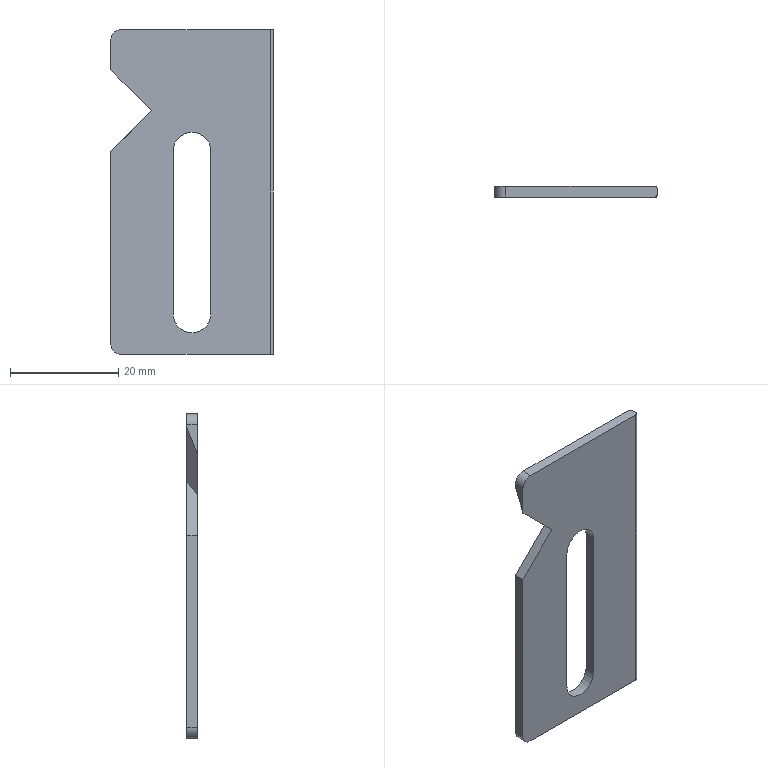Part | SolidWorks | features BaseBody 1 | 1 solid | 18 faces | box 30 x 2 x 60 mm | volume 2939 mm3 | plane 11 | cylinder 7 | commonest cylinder face diameters 7 x3 1 x2 4 x2
STEP:
#1=CARTESIAN_POINT('',(-11.5,0.,-22.5));
#2=VERTEX_POINT('',#1);
#3=CARTESIAN_POINT('',(-15.,0.,-19.));
#4=VERTEX_POINT('',#3);
#5=CARTESIAN_POINT('',(-15.,0.,-22.5));
#6=DIRECTION('',(0.,-1.,0.));
#7=DIRECTION('',(0.,0.,1.));
#8=AXIS2_PLACEMENT_3D('',#5,#6,#7);
#9=CIRCLE('',#8,3.5);
#10=EDGE_CURVE('',#2,#4,#9,.T.);
#11=ORIENTED_EDGE('',*,*,#10,.T.);
#12=CARTESIAN_POINT('',(-15.,2.,-19.));
#13=VERTEX_POINT('',#12);
#14=CARTESIAN_POINT('',(-15.,-8.,-19.));
#15=DIRECTION('',(0.,1.,0.));
#16=VECTOR('',#15,1000.);
#17=LINE('',#14,#16);
#18=EDGE_CURVE('',#4,#13,#17,.T.);
#19=ORIENTED_EDGE('',*,*,#18,.T.);
#20=CARTESIAN_POINT('',(-11.5,2.,-22.5));
#21=VERTEX_POINT('',#20);
#22=CARTESIAN_POINT('',(-15.,2.,-22.5));
#23=DIRECTION('',(0.,-1.,0.));
#24=DIRECTION('',(0.,0.,1.));
#25=AXIS2_PLACEMENT_3D('',#22,#23,#24);
#26=CIRCLE('',#25,3.5);
#27=EDGE_CURVE('',#21,#13,#26,.T.);
#28=ORIENTED_EDGE('',*,*,#27,.F.);
#29=CARTESIAN_POINT('',(-11.5,-8.,-22.5));
#30=DIRECTION('',(0.,1.,0.));
#31=VECTOR('',#30,1000.);
#32=LINE('',#29,#31);
#33=EDGE_CURVE('',#2,#21,#32,.T.);
#34=ORIENTED_EDGE('',*,*,#33,.F.);
#35=EDGE_LOOP('',(#11,#19,#28,#34));
#36=FACE_OUTER_BOUND('',#35,.T.);
#37=CARTESIAN_POINT('',(-15.,-8.,-22.5));
#38=DIRECTION('',(0.,1.,0.));
#39=DIRECTION('',(0.,0.,1.));
#40=AXIS2_PLACEMENT_3D('',#37,#38,#39);
#41=CYLINDRICAL_SURFACE('',#40,3.5);
#42=ADVANCED_FACE('',(#36),#41,.F.);
#43=CARTESIAN_POINT('',(-30.,0.,-22.5));
#44=VERTEX_POINT('',#43);
#45=CARTESIAN_POINT('',(-22.475,0.,-14.975));
#46=VERTEX_POINT('',#45);
#47=CARTESIAN_POINT('',(-30.,0.,-22.5));
#48=DIRECTION('',(0.7071,0.,0.7071));
#49=VECTOR('',#48,1000.);
#50=LINE('',#47,#49);
#51=EDGE_CURVE('',#44,#46,#50,.T.);
#52=ORIENTED_EDGE('',*,*,#51,.F.);
#53=CARTESIAN_POINT('',(-30.,0.,-58.));
#54=VERTEX_POINT('',#53);
#55=CARTESIAN_POINT('',(-30.,0.,-60.));
#56=DIRECTION('',(0.,0.,1.));
#57=VECTOR('',#56,1000.);
#58=LINE('',#55,#57);
#59=EDGE_CURVE('',#54,#44,#58,.T.);
#60=ORIENTED_EDGE('',*,*,#59,.F.);
#61=CARTESIAN_POINT('',(-28.,0.,-60.));
#62=VERTEX_POINT('',#61);
#63=CARTESIAN_POINT('',(-28.,0.,-58.));
#64=DIRECTION('',(0.,1.,0.));
#65=DIRECTION('',(0.,0.,-1.));
#66=AXIS2_PLACEMENT_3D('',#63,#64,#65);
#67=CIRCLE('',#66,2.);
#68=EDGE_CURVE('',#62,#54,#67,.T.);
#69=ORIENTED_EDGE('',*,*,#68,.F.);
#70=CARTESIAN_POINT('',(-0.5,0.,-60.));
#71=VERTEX_POINT('',#70);
#72=CARTESIAN_POINT('',(0.,0.,-60.));
#73=DIRECTION('',(-1.,0.,0.));
#74=VECTOR('',#73,1000.);
#75=LINE('',#72,#74);
#76=EDGE_CURVE('',#71,#62,#75,.T.);
#77=ORIENTED_EDGE('',*,*,#76,.F.);
#78=CARTESIAN_POINT('',(-0.5,0.,0.));
#79=VERTEX_POINT('',#78);
#80=CARTESIAN_POINT('',(-0.5,0.,-60.));
#81=DIRECTION('',(0.,0.,-1.));
#82=VECTOR('',#81,1000.);
#83=LINE('',#80,#82);
#84=EDGE_CURVE('',#79,#71,#83,.T.);
#85=ORIENTED_EDGE('',*,*,#84,.F.);
#86=CARTESIAN_POINT('',(-28.,0.,0.));
#87=VERTEX_POINT('',#86);
#88=CARTESIAN_POINT('',(0.,0.,0.));
#89=DIRECTION('',(1.,0.,0.));
#90=VECTOR('',#89,1000.);
#91=LINE('',#88,#90);
#92=EDGE_CURVE('',#87,#79,#91,.T.);
#93=ORIENTED_EDGE('',*,*,#92,.F.);
#94=CARTESIAN_POINT('',(-30.,0.,-2.));
#95=VERTEX_POINT('',#94);
#96=CARTESIAN_POINT('',(-28.,0.,-2.));
#97=DIRECTION('',(0.,1.,0.));
#98=DIRECTION('',(0.,0.,-1.));
#99=AXIS2_PLACEMENT_3D('',#96,#97,#98);
#100=CIRCLE('',#99,2.);
#101=EDGE_CURVE('',#95,#87,#100,.T.);
#102=ORIENTED_EDGE('',*,*,#101,.F.);
#103=CARTESIAN_POINT('',(-30.,0.,-7.449));
#104=VERTEX_POINT('',#103);
#105=CARTESIAN_POINT('',(-30.,0.,-60.));
#106=DIRECTION('',(0.,0.,1.));
#107=VECTOR('',#106,1000.);
#108=LINE('',#105,#107);
#109=EDGE_CURVE('',#104,#95,#108,.T.);
#110=ORIENTED_EDGE('',*,*,#109,.F.);
#111=CARTESIAN_POINT('',(-22.475,0.,-14.975));
#112=DIRECTION('',(-0.7071,0.,0.7071));
#113=VECTOR('',#112,1000.);
#114=LINE('',#111,#113);
#115=EDGE_CURVE('',#46,#104,#114,.T.);
#116=ORIENTED_EDGE('',*,*,#115,.F.);
#117=EDGE_LOOP('',(#52,#60,#69,#77,#85,#93,#102,#110,#116));
#118=FACE_OUTER_BOUND('',#117,.T.);
#119=CARTESIAN_POINT('',(-18.5,0.,-22.5));
#120=VERTEX_POINT('',#119);
#121=CARTESIAN_POINT('',(-18.5,0.,-52.5));
#122=VERTEX_POINT('',#121);
#123=CARTESIAN_POINT('',(-18.5,0.,-60.));
#124=DIRECTION('',(0.,0.,-1.));
#125=VECTOR('',#124,1000.);
#126=LINE('',#123,#125);
#127=EDGE_CURVE('',#120,#122,#126,.T.);
#128=ORIENTED_EDGE('',*,*,#127,.F.);
#129=CARTESIAN_POINT('',(-15.,0.,-22.5));
#130=DIRECTION('',(0.,-1.,0.));
#131=DIRECTION('',(0.,0.,1.));
#132=AXIS2_PLACEMENT_3D('',#129,#130,#131);
#133=CIRCLE('',#132,3.5);
#134=EDGE_CURVE('',#4,#120,#133,.T.);
#135=ORIENTED_EDGE('',*,*,#134,.F.);
#136=ORIENTED_EDGE('',*,*,#10,.F.);
#137=CARTESIAN_POINT('',(-11.5,0.,-52.5));
#138=VERTEX_POINT('',#137);
#139=CARTESIAN_POINT('',(-11.5,0.,-60.));
#140=DIRECTION('',(0.,0.,1.));
#141=VECTOR('',#140,1000.);
#142=LINE('',#139,#141);
#143=EDGE_CURVE('',#138,#2,#142,.T.);
#144=ORIENTED_EDGE('',*,*,#143,.F.);
#145=CARTESIAN_POINT('',(-15.,0.,-52.5));
#146=DIRECTION('',(0.,-1.,0.));
#147=DIRECTION('',(0.,0.,1.));
#148=AXIS2_PLACEMENT_3D('',#145,#146,#147);
#149=CIRCLE('',#148,3.5);
#150=EDGE_CURVE('',#122,#138,#149,.T.);
#151=ORIENTED_EDGE('',*,*,#150,.F.);
#152=EDGE_LOOP('',(#128,#135,#136,#144,#151));
#153=FACE_BOUND('',#152,.T.);
#154=CARTESIAN_POINT('',(0.,0.,-60.));
#155=DIRECTION('',(0.,1.,0.));
#156=DIRECTION('',(0.,0.,1.));
#157=AXIS2_PLACEMENT_3D('',#154,#155,#156);
#158=PLANE('',#157);
#159=ADVANCED_FACE('',(#118,#153),#158,.F.);
#160=CARTESIAN_POINT('',(-20.025,2.,-12.525));
#161=VERTEX_POINT('',#160);
#162=CARTESIAN_POINT('',(-20.025,2.,-12.525));
#163=DIRECTION('',(-0.6124,-0.5,-0.6124));
#164=VECTOR('',#163,1000.);
#165=LINE('',#162,#164);
#166=EDGE_CURVE('',#161,#46,#165,.T.);
#167=ORIENTED_EDGE('',*,*,#166,.T.);
#168=ORIENTED_EDGE('',*,*,#115,.T.);
#169=CARTESIAN_POINT('',(-30.,2.,-2.55));
#170=VERTEX_POINT('',#169);
#171=CARTESIAN_POINT('',(-30.,-2.645,-13.929));
#172=DIRECTION('',(0.,0.378,0.9258));
#173=VECTOR('',#172,1000.);
#174=LINE('',#171,#173);
#175=EDGE_CURVE('',#104,#170,#174,.T.);
#176=ORIENTED_EDGE('',*,*,#175,.T.);
#177=CARTESIAN_POINT('',(-30.,2.,-2.55));
#178=DIRECTION('',(0.7071,0.,-0.7071));
#179=VECTOR('',#178,1000.);
#180=LINE('',#177,#179);
#181=EDGE_CURVE('',#170,#161,#180,.T.);
#182=ORIENTED_EDGE('',*,*,#181,.T.);
#183=EDGE_LOOP('',(#167,#168,#176,#182));
#184=FACE_OUTER_BOUND('',#183,.T.);
#185=CARTESIAN_POINT('',(-22.5,-0.02073,-15.));
#186=DIRECTION('',(-0.3536,0.866,-0.3536));
#187=DIRECTION('',(0.,0.378,0.9258));
#188=AXIS2_PLACEMENT_3D('',#185,#186,#187);
#189=PLANE('',#188);
#190=ADVANCED_FACE('',(#184),#189,.T.);
#191=CARTESIAN_POINT('',(-30.,2.,-22.5));
#192=VERTEX_POINT('',#191);
#193=CARTESIAN_POINT('',(-30.,10.,-22.5));
#194=DIRECTION('',(0.,1.,0.));
#195=VECTOR('',#194,1000.);
#196=LINE('',#193,#195);
#197=EDGE_CURVE('',#44,#192,#196,.T.);
#198=ORIENTED_EDGE('',*,*,#197,.F.);
#199=ORIENTED_EDGE('',*,*,#51,.T.);
#200=ORIENTED_EDGE('',*,*,#166,.F.);
#201=CARTESIAN_POINT('',(-30.,2.,-22.5));
#202=DIRECTION('',(0.7071,0.,0.7071));
#203=VECTOR('',#202,1000.);
#204=LINE('',#201,#203);
#205=EDGE_CURVE('',#192,#161,#204,.T.);
#206=ORIENTED_EDGE('',*,*,#205,.F.);
#207=EDGE_LOOP('',(#198,#199,#200,#206));
#208=FACE_OUTER_BOUND('',#207,.T.);
#209=CARTESIAN_POINT('',(-30.,10.,-22.5));
#210=DIRECTION('',(0.7071,0.,-0.7071));
#211=DIRECTION('',(-0.7071,0.,-0.7071));
#212=AXIS2_PLACEMENT_3D('',#209,#210,#211);
#213=PLANE('',#212);
#214=ADVANCED_FACE('',(#208),#213,.F.);
#215=CARTESIAN_POINT('',(-30.,2.,-58.));
#216=VERTEX_POINT('',#215);
#217=CARTESIAN_POINT('',(-30.,2.,-58.));
#218=DIRECTION('',(0.,1.,0.));
#219=VECTOR('',#218,1000.);
#220=LINE('',#217,#219);
#221=EDGE_CURVE('',#54,#216,#220,.T.);
#222=ORIENTED_EDGE('',*,*,#221,.F.);
#223=ORIENTED_EDGE('',*,*,#59,.T.);
#224=ORIENTED_EDGE('',*,*,#197,.T.);
#225=CARTESIAN_POINT('',(-30.,2.,0.));
#226=DIRECTION('',(0.,0.,1.));
#227=VECTOR('',#226,1000.);
#228=LINE('',#225,#227);
#229=EDGE_CURVE('',#216,#192,#228,.T.);
#230=ORIENTED_EDGE('',*,*,#229,.F.);
#231=EDGE_LOOP('',(#222,#223,#224,#230));
#232=FACE_OUTER_BOUND('',#231,.T.);
#233=CARTESIAN_POINT('',(-30.,2.,0.));
#234=DIRECTION('',(1.,0.,0.));
#235=DIRECTION('',(0.,0.,-1.));
#236=AXIS2_PLACEMENT_3D('',#233,#234,#235);
#237=PLANE('',#236);
#238=ADVANCED_FACE('',(#232),#237,.F.);
#239=ORIENTED_EDGE('',*,*,#68,.T.);
#240=ORIENTED_EDGE('',*,*,#221,.T.);
#241=CARTESIAN_POINT('',(-28.,2.,-60.));
#242=VERTEX_POINT('',#241);
#243=CARTESIAN_POINT('',(-28.,2.,-58.));
#244=DIRECTION('',(0.,-1.,0.));
#245=DIRECTION('',(0.,0.,-1.));
#246=AXIS2_PLACEMENT_3D('',#243,#244,#245);
#247=CIRCLE('',#246,2.);
#248=EDGE_CURVE('',#216,#242,#247,.T.);
#249=ORIENTED_EDGE('',*,*,#248,.T.);
#250=CARTESIAN_POINT('',(-28.,2.,-60.));
#251=DIRECTION('',(0.,-1.,0.));
#252=VECTOR('',#251,1000.);
#253=LINE('',#250,#252);
#254=EDGE_CURVE('',#242,#62,#253,.T.);
#255=ORIENTED_EDGE('',*,*,#254,.T.);
#256=EDGE_LOOP('',(#239,#240,#249,#255));
#257=FACE_OUTER_BOUND('',#256,.T.);
#258=CARTESIAN_POINT('',(-28.,2.,-58.));
#259=DIRECTION('',(0.,-1.,0.));
#260=DIRECTION('',(0.,0.,-1.));
#261=AXIS2_PLACEMENT_3D('',#258,#259,#260);
#262=CYLINDRICAL_SURFACE('',#261,2.);
#263=ADVANCED_FACE('',(#257),#262,.T.);
#264=ORIENTED_EDGE('',*,*,#254,.F.);
#265=CARTESIAN_POINT('',(-0.5,2.,-60.));
#266=VERTEX_POINT('',#265);
#267=CARTESIAN_POINT('',(0.,2.,-60.));
#268=DIRECTION('',(-1.,0.,0.));
#269=VECTOR('',#268,1000.);
#270=LINE('',#267,#269);
#271=EDGE_CURVE('',#266,#242,#270,.T.);
#272=ORIENTED_EDGE('',*,*,#271,.F.);
#273=CARTESIAN_POINT('',(0.,1.5,-60.));
#274=VERTEX_POINT('',#273);
#275=CARTESIAN_POINT('',(-0.5,1.5,-60.));
#276=DIRECTION('',(0.,0.,1.));
#277=DIRECTION('',(1.,0.,0.));
#278=AXIS2_PLACEMENT_3D('',#275,#276,#277);
#279=CIRCLE('',#278,0.5);
#280=EDGE_CURVE('',#274,#266,#279,.T.);
#281=ORIENTED_EDGE('',*,*,#280,.F.);
#282=CARTESIAN_POINT('',(0.,0.5,-60.));
#283=VERTEX_POINT('',#282);
#284=CARTESIAN_POINT('',(0.,2.,-60.));
#285=DIRECTION('',(0.,-1.,0.));
#286=VECTOR('',#285,1000.);
#287=LINE('',#284,#286);
#288=EDGE_CURVE('',#274,#283,#287,.T.);
#289=ORIENTED_EDGE('',*,*,#288,.T.);
#290=CARTESIAN_POINT('',(-0.5,0.5,-60.));
#291=DIRECTION('',(0.,0.,1.));
#292=DIRECTION('',(-1.,0.,0.));
#293=AXIS2_PLACEMENT_3D('',#290,#291,#292);
#294=CIRCLE('',#293,0.5);
#295=EDGE_CURVE('',#71,#283,#294,.T.);
#296=ORIENTED_EDGE('',*,*,#295,.F.);
#297=ORIENTED_EDGE('',*,*,#76,.T.);
#298=EDGE_LOOP('',(#264,#272,#281,#289,#296,#297));
#299=FACE_OUTER_BOUND('',#298,.T.);
#300=CARTESIAN_POINT('',(0.,2.,-60.));
#301=DIRECTION('',(0.,0.,1.));
#302=DIRECTION('',(1.,0.,0.));
#303=AXIS2_PLACEMENT_3D('',#300,#301,#302);
#304=PLANE('',#303);
#305=ADVANCED_FACE('',(#299),#304,.F.);
#306=ORIENTED_EDGE('',*,*,#295,.T.);
#307=CARTESIAN_POINT('',(0.,0.5,0.));
#308=VERTEX_POINT('',#307);
#309=CARTESIAN_POINT('',(0.,0.5,0.));
#310=DIRECTION('',(0.,0.,1.));
#311=VECTOR('',#310,1000.);
#312=LINE('',#309,#311);
#313=EDGE_CURVE('',#283,#308,#312,.T.);
#314=ORIENTED_EDGE('',*,*,#313,.T.);
#315=CARTESIAN_POINT('',(-0.5,0.5,0.));
#316=DIRECTION('',(0.,0.,-1.));
#317=DIRECTION('',(-1.,0.,0.));
#318=AXIS2_PLACEMENT_3D('',#315,#316,#317);
#319=CIRCLE('',#318,0.5);
#320=EDGE_CURVE('',#308,#79,#319,.T.);
#321=ORIENTED_EDGE('',*,*,#320,.T.);
#322=ORIENTED_EDGE('',*,*,#84,.T.);
#323=EDGE_LOOP('',(#306,#314,#321,#322));
#324=FACE_OUTER_BOUND('',#323,.T.);
#325=CARTESIAN_POINT('',(-0.5,0.5,0.));
#326=DIRECTION('',(0.,0.,-1.));
#327=DIRECTION('',(-1.,0.,0.));
#328=AXIS2_PLACEMENT_3D('',#325,#326,#327);
#329=CYLINDRICAL_SURFACE('',#328,0.5);
#330=ADVANCED_FACE('',(#324),#329,.T.);
#331=CARTESIAN_POINT('',(-28.,2.,0.));
#332=VERTEX_POINT('',#331);
#333=CARTESIAN_POINT('',(-28.,2.,0.));
#334=DIRECTION('',(0.,1.,0.));
#335=VECTOR('',#334,1000.);
#336=LINE('',#333,#335);
#337=EDGE_CURVE('',#87,#332,#336,.T.);
#338=ORIENTED_EDGE('',*,*,#337,.F.);
#339=ORIENTED_EDGE('',*,*,#92,.T.);
#340=ORIENTED_EDGE('',*,*,#320,.F.);
#341=CARTESIAN_POINT('',(0.,1.5,0.));
#342=VERTEX_POINT('',#341);
#343=CARTESIAN_POINT('',(0.,2.,0.));
#344=DIRECTION('',(0.,-1.,0.));
#345=VECTOR('',#344,1000.);
#346=LINE('',#343,#345);
#347=EDGE_CURVE('',#342,#308,#346,.T.);
#348=ORIENTED_EDGE('',*,*,#347,.F.);
#349=CARTESIAN_POINT('',(-0.5,2.,0.));
#350=VERTEX_POINT('',#349);
#351=CARTESIAN_POINT('',(-0.5,1.5,0.));
#352=DIRECTION('',(0.,0.,-1.));
#353=DIRECTION('',(1.,0.,0.));
#354=AXIS2_PLACEMENT_3D('',#351,#352,#353);
#355=CIRCLE('',#354,0.5);
#356=EDGE_CURVE('',#350,#342,#355,.T.);
#357=ORIENTED_EDGE('',*,*,#356,.F.);
#358=CARTESIAN_POINT('',(0.,2.,0.));
#359=DIRECTION('',(1.,0.,0.));
#360=VECTOR('',#359,1000.);
#361=LINE('',#358,#360);
#362=EDGE_CURVE('',#332,#350,#361,.T.);
#363=ORIENTED_EDGE('',*,*,#362,.F.);
#364=EDGE_LOOP('',(#338,#339,#340,#348,#357,#363));
#365=FACE_OUTER_BOUND('',#364,.T.);
#366=CARTESIAN_POINT('',(0.,2.,0.));
#367=DIRECTION('',(0.,0.,-1.));
#368=DIRECTION('',(-1.,0.,0.));
#369=AXIS2_PLACEMENT_3D('',#366,#367,#368);
#370=PLANE('',#369);
#371=ADVANCED_FACE('',(#365),#370,.F.);
#372=ORIENTED_EDGE('',*,*,#101,.T.);
#373=ORIENTED_EDGE('',*,*,#337,.T.);
#374=CARTESIAN_POINT('',(-30.,2.,-2.));
#375=VERTEX_POINT('',#374);
#376=CARTESIAN_POINT('',(-28.,2.,-2.));
#377=DIRECTION('',(0.,-1.,0.));
#378=DIRECTION('',(0.,0.,-1.));
#379=AXIS2_PLACEMENT_3D('',#376,#377,#378);
#380=CIRCLE('',#379,2.);
#381=EDGE_CURVE('',#332,#375,#380,.T.);
#382=ORIENTED_EDGE('',*,*,#381,.T.);
#383=CARTESIAN_POINT('',(-30.,2.,-2.));
#384=DIRECTION('',(0.,-1.,0.));
#385=VECTOR('',#384,1000.);
#386=LINE('',#383,#385);
#387=EDGE_CURVE('',#375,#95,#386,.T.);
#388=ORIENTED_EDGE('',*,*,#387,.T.);
#389=EDGE_LOOP('',(#372,#373,#382,#388));
#390=FACE_OUTER_BOUND('',#389,.T.);
#391=CARTESIAN_POINT('',(-28.,2.,-2.));
#392=DIRECTION('',(0.,-1.,0.));
#393=DIRECTION('',(0.,0.,-1.));
#394=AXIS2_PLACEMENT_3D('',#391,#392,#393);
#395=CYLINDRICAL_SURFACE('',#394,2.);
#396=ADVANCED_FACE('',(#390),#395,.T.);
#397=ORIENTED_EDGE('',*,*,#175,.F.);
#398=ORIENTED_EDGE('',*,*,#109,.T.);
#399=ORIENTED_EDGE('',*,*,#387,.F.);
#400=CARTESIAN_POINT('',(-30.,2.,0.));
#401=DIRECTION('',(0.,0.,1.));
#402=VECTOR('',#401,1000.);
#403=LINE('',#400,#402);
#404=EDGE_CURVE('',#170,#375,#403,.T.);
#405=ORIENTED_EDGE('',*,*,#404,.F.);
#406=EDGE_LOOP('',(#397,#398,#399,#405));
#407=FACE_OUTER_BOUND('',#406,.T.);
#408=CARTESIAN_POINT('',(-30.,2.,0.));
#409=DIRECTION('',(1.,0.,0.));
#410=DIRECTION('',(0.,0.,-1.));
#411=AXIS2_PLACEMENT_3D('',#408,#409,#410);
#412=PLANE('',#411);
#413=ADVANCED_FACE('',(#407),#412,.F.);
#414=CARTESIAN_POINT('',(-18.5,2.,-22.5));
#415=VERTEX_POINT('',#414);
#416=CARTESIAN_POINT('',(-18.5,2.,-52.5));
#417=VERTEX_POINT('',#416);
#418=CARTESIAN_POINT('',(-18.5,2.,-22.5));
#419=DIRECTION('',(0.,0.,-1.));
#420=VECTOR('',#419,1000.);
#421=LINE('',#418,#420);
#422=EDGE_CURVE('',#415,#417,#421,.T.);
#423=ORIENTED_EDGE('',*,*,#422,.F.);
#424=CARTESIAN_POINT('',(-18.5,-8.,-22.5));
#425=DIRECTION('',(0.,1.,0.));
#426=VECTOR('',#425,1000.);
#427=LINE('',#424,#426);
#428=EDGE_CURVE('',#120,#415,#427,.T.);
#429=ORIENTED_EDGE('',*,*,#428,.F.);
#430=ORIENTED_EDGE('',*,*,#127,.T.);
#431=CARTESIAN_POINT('',(-18.5,-8.,-52.5));
#432=DIRECTION('',(0.,-1.,0.));
#433=VECTOR('',#432,1000.);
#434=LINE('',#431,#433);
#435=EDGE_CURVE('',#417,#122,#434,.T.);
#436=ORIENTED_EDGE('',*,*,#435,.F.);
#437=EDGE_LOOP('',(#423,#429,#430,#436));
#438=FACE_OUTER_BOUND('',#437,.T.);
#439=CARTESIAN_POINT('',(-18.5,-8.,-22.5));
#440=DIRECTION('',(-1.,0.,0.));
#441=DIRECTION('',(0.,0.,1.));
#442=AXIS2_PLACEMENT_3D('',#439,#440,#441);
#443=PLANE('',#442);
#444=ADVANCED_FACE('',(#438),#443,.F.);
#445=ORIENTED_EDGE('',*,*,#18,.F.);
#446=ORIENTED_EDGE('',*,*,#134,.T.);
#447=ORIENTED_EDGE('',*,*,#428,.T.);
#448=CARTESIAN_POINT('',(-15.,2.,-22.5));
#449=DIRECTION('',(0.,-1.,0.));
#450=DIRECTION('',(0.,0.,1.));
#451=AXIS2_PLACEMENT_3D('',#448,#449,#450);
#452=CIRCLE('',#451,3.5);
#453=EDGE_CURVE('',#13,#415,#452,.T.);
#454=ORIENTED_EDGE('',*,*,#453,.F.);
#455=EDGE_LOOP('',(#445,#446,#447,#454));
#456=FACE_OUTER_BOUND('',#455,.T.);
#457=CARTESIAN_POINT('',(-15.,-8.,-22.5));
#458=DIRECTION('',(0.,1.,0.));
#459=DIRECTION('',(0.,0.,1.));
#460=AXIS2_PLACEMENT_3D('',#457,#458,#459);
#461=CYLINDRICAL_SURFACE('',#460,3.5);
#462=ADVANCED_FACE('',(#456),#461,.F.);
#463=CARTESIAN_POINT('',(-11.5,2.,-52.5));
#464=VERTEX_POINT('',#463);
#465=CARTESIAN_POINT('',(-11.5,2.,-22.5));
#466=DIRECTION('',(0.,0.,1.));
#467=VECTOR('',#466,1000.);
#468=LINE('',#465,#467);
#469=EDGE_CURVE('',#464,#21,#468,.T.);
#470=ORIENTED_EDGE('',*,*,#469,.F.);
#471=CARTESIAN_POINT('',(-11.5,-8.,-52.5));
#472=DIRECTION('',(0.,1.,0.));
#473=VECTOR('',#472,1000.);
#474=LINE('',#471,#473);
#475=EDGE_CURVE('',#138,#464,#474,.T.);
#476=ORIENTED_EDGE('',*,*,#475,.F.);
#477=ORIENTED_EDGE('',*,*,#143,.T.);
#478=ORIENTED_EDGE('',*,*,#33,.T.);
#479=EDGE_LOOP('',(#470,#476,#477,#478));
#480=FACE_OUTER_BOUND('',#479,.T.);
#481=CARTESIAN_POINT('',(-11.5,-8.,-22.5));
#482=DIRECTION('',(1.,0.,0.));
#483=DIRECTION('',(0.,0.,-1.));
#484=AXIS2_PLACEMENT_3D('',#481,#482,#483);
#485=PLANE('',#484);
#486=ADVANCED_FACE('',(#480),#485,.F.);
#487=CARTESIAN_POINT('',(-15.,2.,-52.5));
#488=DIRECTION('',(0.,-1.,0.));
#489=DIRECTION('',(0.,0.,1.));
#490=AXIS2_PLACEMENT_3D('',#487,#488,#489);
#491=CIRCLE('',#490,3.5);
#492=EDGE_CURVE('',#417,#464,#491,.T.);
#493=ORIENTED_EDGE('',*,*,#492,.F.);
#494=ORIENTED_EDGE('',*,*,#435,.T.);
#495=ORIENTED_EDGE('',*,*,#150,.T.);
#496=ORIENTED_EDGE('',*,*,#475,.T.);
#497=EDGE_LOOP('',(#493,#494,#495,#496));
#498=FACE_OUTER_BOUND('',#497,.T.);
#499=CARTESIAN_POINT('',(-15.,-8.,-52.5));
#500=DIRECTION('',(0.,1.,0.));
#501=DIRECTION('',(0.,0.,1.));
#502=AXIS2_PLACEMENT_3D('',#499,#500,#501);
#503=CYLINDRICAL_SURFACE('',#502,3.5);
#504=ADVANCED_FACE('',(#498),#503,.F.);
#505=ORIENTED_EDGE('',*,*,#469,.T.);
#506=ORIENTED_EDGE('',*,*,#27,.T.);
#507=ORIENTED_EDGE('',*,*,#453,.T.);
#508=ORIENTED_EDGE('',*,*,#422,.T.);
#509=ORIENTED_EDGE('',*,*,#492,.T.);
#510=EDGE_LOOP('',(#505,#506,#507,#508,#509));
#511=FACE_BOUND('',#510,.T.);
#512=ORIENTED_EDGE('',*,*,#248,.F.);
#513=ORIENTED_EDGE('',*,*,#229,.T.);
#514=ORIENTED_EDGE('',*,*,#205,.T.);
#515=ORIENTED_EDGE('',*,*,#181,.F.);
#516=ORIENTED_EDGE('',*,*,#404,.T.);
#517=ORIENTED_EDGE('',*,*,#381,.F.);
#518=ORIENTED_EDGE('',*,*,#362,.T.);
#519=CARTESIAN_POINT('',(-0.5,2.,-60.));
#520=DIRECTION('',(0.,0.,-1.));
#521=VECTOR('',#520,1000.);
#522=LINE('',#519,#521);
#523=EDGE_CURVE('',#350,#266,#522,.T.);
#524=ORIENTED_EDGE('',*,*,#523,.T.);
#525=ORIENTED_EDGE('',*,*,#271,.T.);
#526=EDGE_LOOP('',(#512,#513,#514,#515,#516,#517,#518,#524,#525));
#527=FACE_OUTER_BOUND('',#526,.T.);
#528=CARTESIAN_POINT('',(0.,2.,-60.));
#529=DIRECTION('',(0.,1.,0.));
#530=DIRECTION('',(0.,0.,1.));
#531=AXIS2_PLACEMENT_3D('',#528,#529,#530);
#532=PLANE('',#531);
#533=ADVANCED_FACE('',(#511,#527),#532,.T.);
#534=ORIENTED_EDGE('',*,*,#313,.F.);
#535=ORIENTED_EDGE('',*,*,#288,.F.);
#536=CARTESIAN_POINT('',(0.,1.5,0.));
#537=DIRECTION('',(0.,0.,-1.));
#538=VECTOR('',#537,1000.);
#539=LINE('',#536,#538);
#540=EDGE_CURVE('',#342,#274,#539,.T.);
#541=ORIENTED_EDGE('',*,*,#540,.F.);
#542=ORIENTED_EDGE('',*,*,#347,.T.);
#543=EDGE_LOOP('',(#534,#535,#541,#542));
#544=FACE_OUTER_BOUND('',#543,.T.);
#545=CARTESIAN_POINT('',(0.,2.,0.));
#546=DIRECTION('',(-1.,0.,0.));
#547=DIRECTION('',(0.,0.,1.));
#548=AXIS2_PLACEMENT_3D('',#545,#546,#547);
#549=PLANE('',#548);
#550=ADVANCED_FACE('',(#544),#549,.F.);
#551=ORIENTED_EDGE('',*,*,#280,.T.);
#552=ORIENTED_EDGE('',*,*,#523,.F.);
#553=ORIENTED_EDGE('',*,*,#356,.T.);
#554=ORIENTED_EDGE('',*,*,#540,.T.);
#555=EDGE_LOOP('',(#551,#552,#553,#554));
#556=FACE_OUTER_BOUND('',#555,.T.);
#557=CARTESIAN_POINT('',(-0.5,1.5,-60.));
#558=DIRECTION('',(0.,0.,1.));
#559=DIRECTION('',(1.,0.,0.));
#560=AXIS2_PLACEMENT_3D('',#557,#558,#559);
#561=CYLINDRICAL_SURFACE('',#560,0.5);
#562=ADVANCED_FACE('',(#556),#561,.T.);
#563=CLOSED_SHELL('',(#42,#159,#190,#214,#238,#263,#305,#330,#371,#396,#413,#444,#462,#486,#504,#533,#550,#562));
#564=MANIFOLD_SOLID_BREP('',#563);
#565=CARTESIAN_POINT('',(0.,0.,0.));
#566=DIRECTION('',(0.,0.,1.));
#567=DIRECTION('',(1.,0.,0.));
#568=AXIS2_PLACEMENT_3D('',#565,#566,#567);
#569=(LENGTH_UNIT()NAMED_UNIT(*)SI_UNIT(.MILLI.,.METRE.));
#570=UNCERTAINTY_MEASURE_WITH_UNIT(LENGTH_MEASURE(0.00001),#569,'','');
#571=(NAMED_UNIT(*)PLANE_ANGLE_UNIT()SI_UNIT($,.RADIAN.));
#572=(NAMED_UNIT(*)SI_UNIT($,.STERADIAN.)SOLID_ANGLE_UNIT());
#573=(GEOMETRIC_REPRESENTATION_CONTEXT(3)GLOBAL_UNCERTAINTY_ASSIGNED_CONTEXT((#570))GLOBAL_UNIT_ASSIGNED_CONTEXT((#569,#571,#572))REPRESENTATION_CONTEXT('',''));
#574=ADVANCED_BREP_SHAPE_REPRESENTATION('',(#564,#568),#573);